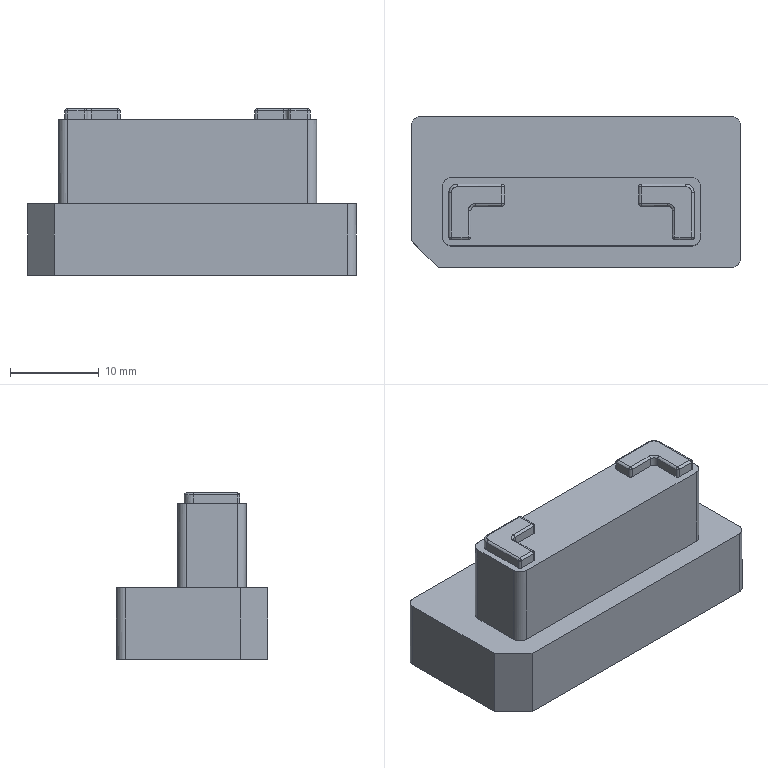NC program | PowerMill | posted with a generic post | part box 37 x 17 x 18.689 mm
Lines 3504 to 4371 of 30982:
N3601 M6
N3602 S18000 M03
N3603 G00 G90 X0.0 Y0.0
N3604 G43 Z9.7991 H2
N3605
N3606 G05 P10000 R4
N3607 X-17.264 Y-4.1178
N3608 Z0.7955
N3609 G01 Z-0.4045 F3600.0
N3610 X-17.2443 Y-4.1277 F6000.0
N3611 G03 X-16.9786 Y-4.0391 I0.0886 J0.1771
N3612 G01 X-16.3013 Y-2.6843
N3613 X-16.3014 Y-0.244
N3614 X-16.2791 Y0.244
N3615 X-16.1772 Y0.7321
N3616 X-15.9859 Y1.2201
N3617 X-15.6795 Y1.7082
N3618 X-15.2056 Y2.1962
N3619 X-14.6416 Y2.5601
N3620 X-14.1535 Y2.7484
N3621 X-13.6655 Y2.8465
N3622 X-13.1774 Y2.8715
N3623 X-8.2969 Y2.871
N3624 X-7.8088 Y2.8049
N3625 X-7.3208 Y2.6313
N3626 X-6.8327 Y2.3035
N3627 X-6.7176 Y2.1962
N3628 X-6.3488 Y1.7082
N3629 X-6.1463 Y1.2201
N3630 X-6.06 Y0.7321
N3631 X-6.0548 Y-1.2201
N3632 X-6.0876 Y-1.7082
N3633 X-6.2286 Y-2.1962
N3634 X-6.3447 Y-2.4359
N3635 X-6.5053 Y-2.6843
N3636 X-6.8327 Y-3.0394
N3637 X-7.0002 Y-3.1723
N3638 X-7.3208 Y-3.3669
N3639 X-7.8088 Y-3.5431
N3640 X-8.2969 Y-3.606
N3641 X-9.6235 Y-3.6064
N3642 G03 X-9.8185 Y-3.7754 I-0.0025 J-0.1942
N3643 G01 X-9.8234 Y-3.8064
N3644 X-9.8238 Y-5.1246
N3645 X-9.8882 Y-5.6126
N3646 X-10.0595 Y-6.1007
N3647 X-10.2491 Y-6.4163
N3648 X-10.3841 Y-6.5887
N3649 X-10.7372 Y-6.9154
N3650 X-10.9788 Y-7.0768
N3651 X-11.2252 Y-7.1978
N3652 X-11.7133 Y-7.3359
N3653 X-12.2013 Y-7.3752
N3654 X-14.1535 Y-7.3707
N3655 X-14.6416 Y-7.288
N3656 X-15.1461 Y-7.0768
N3657 X-15.6177 Y-6.7207
N3658 X-15.7419 Y-6.5887
N3659 X-16.0662 Y-6.1007
N3660 X-16.2402 Y-5.6126
N3661 X-16.3012 Y-5.1246
N3662 X-16.3013 Y-2.6843
N3663 X-17.264 Y-4.1178 Z-0.598
N3664 X-17.2443 Y-4.1277
N3665 G03 X-16.9787 Y-4.0391 I0.0885 J0.1771
N3666 G01 X-16.3013 Y-2.6843
N3667 X-16.3014 Y-0.244
N3668 X-16.2792 Y0.244
N3669 X-16.1773 Y0.7321
N3670 X-15.9859 Y1.2201
N3671 X-15.6795 Y1.7082
N3672 X-15.2056 Y2.1962
N3673 X-14.6416 Y2.5602
N3674 X-14.1535 Y2.7485
N3675 X-13.6655 Y2.8465
N3676 X-13.1774 Y2.8715
N3677 X-8.2969 Y2.871
N3678 X-7.8088 Y2.8049
N3679 X-7.3208 Y2.6314
N3680 X-6.8327 Y2.3035
N3681 X-6.7176 Y2.1962
N3682 X-6.3488 Y1.7082
N3683 X-6.1463 Y1.2201
N3684 X-6.06 Y0.7321
N3685 X-6.0548 Y-1.2201
N3686 X-6.0876 Y-1.7082
N3687 X-6.2286 Y-2.1962
N3688 X-6.3447 Y-2.436
N3689 X-6.5053 Y-2.6843
N3690 X-6.8327 Y-3.0394
N3691 X-7.0002 Y-3.1723
N3692 X-7.3208 Y-3.367
N3693 X-7.8088 Y-3.5432
N3694 X-8.2969 Y-3.6061
N3695 X-9.6235 Y-3.6064
N3696 G03 X-9.8185 Y-3.7754 I-0.0025 J-0.1942
N3697 G01 X-9.8234 Y-3.8064
N3698 X-9.8238 Y-5.1246
N3699 X-9.8882 Y-5.6126
N3700 X-10.0595 Y-6.1007
N3701 X-10.2491 Y-6.4163
N3702 X-10.3841 Y-6.5887
N3703 X-10.7372 Y-6.9154
N3704 X-10.9788 Y-7.0768
N3705 X-11.2252 Y-7.1978
N3706 X-11.7133 Y-7.3359
N3707 X-12.2013 Y-7.3752
N3708 X-14.1535 Y-7.3708
N3709 X-14.6416 Y-7.288
N3710 X-15.1461 Y-7.0768
N3711 X-15.6177 Y-6.7208
N3712 X-15.742 Y-6.5887
N3713 X-16.0662 Y-6.1007
N3714 X-16.2402 Y-5.6126
N3715 X-16.3012 Y-5.1246
N3716 X-16.3013 Y-2.6843
N3717 X-17.264 Y-4.1178 Z-0.7914
N3718 X-17.2443 Y-4.1277
N3719 G03 X-16.9787 Y-4.0391 I0.0885 J0.1771
N3720 G01 X-16.3014 Y-2.6843
N3721 X-16.3015 Y-0.244
N3722 X-16.2793 Y0.244
N3723 X-16.1773 Y0.7321
N3724 X-15.9859 Y1.2201
N3725 X-15.6795 Y1.7082
N3726 X-15.2056 Y2.1962
N3727 X-14.6416 Y2.5602
N3728 X-14.1535 Y2.7485
N3729 X-13.6655 Y2.8465
N3730 X-13.1774 Y2.8715
N3731 X-8.2969 Y2.8711
N3732 X-7.8088 Y2.8049
N3733 X-7.3208 Y2.6314
N3734 X-6.8327 Y2.3035
N3735 X-6.7176 Y2.1962
N3736 X-6.3487 Y1.7082
N3737 X-6.1463 Y1.2201
N3738 X-6.06 Y0.7321
N3739 X-6.0547 Y-1.2201
N3740 X-6.0875 Y-1.7082
N3741 X-6.2285 Y-2.1962
N3742 X-6.3447 Y-2.436
N3743 X-6.5053 Y-2.6843
N3744 X-6.8327 Y-3.0394
N3745 X-7.0002 Y-3.1723
N3746 X-7.3208 Y-3.367
N3747 X-7.8088 Y-3.5432
N3748 X-8.2969 Y-3.6061
N3749 X-9.6235 Y-3.6065
N3750 G03 X-9.8185 Y-3.7754 I-0.0025 J-0.1941
N3751 G01 X-9.8234 Y-3.8064
N3752 X-9.8237 Y-5.1246
N3753 X-9.8882 Y-5.6126
N3754 X-10.0594 Y-6.1007
N3755 X-10.2491 Y-6.4163
N3756 X-10.3841 Y-6.5887
N3757 X-10.7372 Y-6.9154
N3758 X-10.9788 Y-7.0768
N3759 X-11.2252 Y-7.1979
N3760 X-11.7133 Y-7.3359
N3761 X-12.2013 Y-7.3752
N3762 X-14.1535 Y-7.3708
N3763 X-14.6416 Y-7.288
N3764 X-15.1461 Y-7.0768
N3765 X-15.6177 Y-6.7208
N3766 X-15.742 Y-6.5887
N3767 X-16.0662 Y-6.1007
N3768 X-16.2402 Y-5.6126
N3769 X-16.3012 Y-5.1246
N3770 X-16.3014 Y-2.6843
N3771 X-17.264 Y-4.1178 Z-0.9849
N3772 X-17.2443 Y-4.1277
N3773 G03 X-16.9787 Y-4.0391 I0.0885 J0.1771
N3774 G01 X-16.3014 Y-2.6843
N3775 X-16.3015 Y-0.244
N3776 X-16.2795 Y0.244
N3777 X-16.1773 Y0.7321
N3778 X-15.986 Y1.2201
N3779 X-15.6795 Y1.7082
N3780 X-15.2056 Y2.1962
N3781 X-14.6416 Y2.5602
N3782 X-14.1535 Y2.7485
N3783 X-13.6655 Y2.8465
N3784 X-13.1774 Y2.8716
N3785 X-8.2969 Y2.8711
N3786 X-7.8088 Y2.8049
N3787 X-7.3208 Y2.6314
N3788 X-6.8327 Y2.3036
N3789 X-6.7176 Y2.1962
N3790 X-6.3487 Y1.7082
N3791 X-6.1462 Y1.2201
N3792 X-6.06 Y0.7321
N3793 X-6.0547 Y-1.2201
N3794 X-6.0875 Y-1.7082
N3795 X-6.2285 Y-2.1962
N3796 X-6.3447 Y-2.436
N3797 X-6.5053 Y-2.6843
N3798 X-6.8327 Y-3.0395
N3799 X-7.0001 Y-3.1723
N3800 X-7.3208 Y-3.367
N3801 X-7.8088 Y-3.5432
N3802 X-8.2969 Y-3.6061
N3803 X-9.6235 Y-3.6065
N3804 G03 X-9.8185 Y-3.7754 I-0.0025 J-0.1941
N3805 G01 X-9.8234 Y-3.8064
N3806 X-9.8237 Y-5.1246
N3807 X-9.8882 Y-5.6126
N3808 X-10.0594 Y-6.1007
N3809 X-10.2491 Y-6.4163
N3810 X-10.384 Y-6.5887
N3811 X-10.7372 Y-6.9154
N3812 X-10.9788 Y-7.0768
N3813 X-11.2252 Y-7.1979
N3814 X-11.7133 Y-7.336
N3815 X-12.2013 Y-7.3752
N3816 X-14.1535 Y-7.3708
N3817 X-14.6416 Y-7.2881
N3818 X-15.1461 Y-7.0768
N3819 X-15.6177 Y-6.7208
N3820 X-15.742 Y-6.5887
N3821 X-16.0663 Y-6.1007
N3822 X-16.2403 Y-5.6126
N3823 X-16.3013 Y-5.1246
N3824 X-16.3014 Y-2.6843
N3825 X-17.264 Y-4.1178 Z-1.1784
N3826 X-17.2444 Y-4.1276
N3827 G03 X-16.9787 Y-4.0391 I0.0886 J0.1771
N3828 G01 X-16.3014 Y-2.6843
N3829 X-16.3015 Y-0.244
N3830 X-16.2796 Y0.244
N3831 X-16.1773 Y0.7321
N3832 X-15.986 Y1.2201
N3833 X-15.6796 Y1.7082
N3834 X-15.2056 Y2.1962
N3835 X-14.6416 Y2.5602
N3836 X-14.1535 Y2.7485
N3837 X-13.6655 Y2.8466
N3838 X-13.1774 Y2.8716
N3839 X-8.2969 Y2.8711
N3840 X-7.8088 Y2.805
N3841 X-7.3208 Y2.6314
N3842 X-6.8327 Y2.3036
N3843 X-6.7175 Y2.1962
N3844 X-6.3487 Y1.7082
N3845 X-6.1462 Y1.2201
N3846 X-6.06 Y0.7321
N3847 X-6.0547 Y-1.2201
N3848 X-6.0875 Y-1.7082
N3849 X-6.2285 Y-2.1962
N3850 X-6.3447 Y-2.436
N3851 X-6.5052 Y-2.6843
N3852 X-6.8327 Y-3.0395
N3853 X-7.0001 Y-3.1723
N3854 X-7.3208 Y-3.367
N3855 X-7.8088 Y-3.5432
N3856 X-8.2969 Y-3.6061
N3857 X-9.6235 Y-3.6065
N3858 G03 X-9.8185 Y-3.7754 I-0.0025 J-0.1941
N3859 G01 X-9.8234 Y-3.8064
N3860 X-9.8237 Y-5.1246
N3861 X-9.8882 Y-5.6126
N3862 X-10.0594 Y-6.1007
N3863 X-10.2491 Y-6.4163
N3864 X-10.384 Y-6.5887
N3865 X-10.7372 Y-6.9155
N3866 X-10.9788 Y-7.0768
N3867 X-11.2252 Y-7.1979
N3868 X-11.7133 Y-7.336
N3869 X-12.2013 Y-7.3753
N3870 X-14.1535 Y-7.3708
N3871 X-14.6416 Y-7.2881
N3872 X-15.1462 Y-7.0768
N3873 X-15.6177 Y-6.7208
N3874 X-15.742 Y-6.5887
N3875 X-16.0663 Y-6.1007
N3876 X-16.2403 Y-5.6126
N3877 X-16.3013 Y-5.1246
N3878 X-16.3014 Y-2.6843
N3879 X-17.3042 Y-4.1981 Z-1.3719
N3880 X-17.2845 Y-4.208
N3881 G03 X-17.0189 Y-4.1194 I0.0885 J0.1771
N3882 G01 X-16.3014 Y-2.6843
N3883 X-16.3015 Y-0.244
N3884 X-16.2796 Y0.244
N3885 X-16.1774 Y0.7321
N3886 X-15.986 Y1.2201
N3887 X-15.6796 Y1.7082
N3888 X-15.2057 Y2.1962
N3889 X-14.6416 Y2.5602
N3890 X-14.1535 Y2.7485
N3891 X-13.6655 Y2.8466
N3892 X-13.1774 Y2.8716
N3893 X-8.2969 Y2.8711
N3894 X-7.8088 Y2.805
N3895 X-7.3208 Y2.6314
N3896 X-6.8327 Y2.3036
N3897 X-6.7175 Y2.1962
N3898 X-6.3487 Y1.7082
N3899 X-6.1462 Y1.2201
N3900 X-6.0599 Y0.7321
N3901 X-6.0547 Y-1.2201
N3902 X-6.0875 Y-1.7082
N3903 X-6.2285 Y-2.1962
N3904 X-6.3447 Y-2.4361
N3905 X-6.5052 Y-2.6843
N3906 X-6.8327 Y-3.0395
N3907 X-7.0001 Y-3.1723
N3908 X-7.3208 Y-3.3671
N3909 X-7.8088 Y-3.5433
N3910 X-8.2969 Y-3.6061
N3911 X-9.6235 Y-3.6065
N3912 G03 X-9.8234 Y-3.8064 I0.0001 J-0.2
N3913 G01 X-9.8237 Y-5.1246
N3914 X-9.8881 Y-5.6126
N3915 X-10.0594 Y-6.1007
N3916 X-10.2491 Y-6.4164
N3917 X-10.384 Y-6.5887
N3918 X-10.7372 Y-6.9155
N3919 X-10.9787 Y-7.0768
N3920 X-11.2252 Y-7.1979
N3921 X-11.7133 Y-7.336
N3922 X-12.2013 Y-7.3753
N3923 X-14.1535 Y-7.3709
N3924 X-14.6416 Y-7.2881
N3925 X-15.1296 Y-7.0861
N3926 X-15.1378 Y-7.0812
N3927 X-15.1461 Y-7.0767
N3928 X-15.6045 Y-6.7307
N3929 X-15.6177 Y-6.7208
N3930 X-15.742 Y-6.5887
N3931 X-16.0663 Y-6.1007
N3932 X-16.2403 Y-5.6126
N3933 X-16.3013 Y-5.1246
N3934 X-16.3014 Y-2.6843
N3935 G00 Z3.7955
N3936 G01 X4.2528 Y-2.3244 F10000.0
N3937 G00 Z0.7955
N3938 G01 Z-0.4045 F3600.0
N3939 X4.2725 Y-2.3343 F6000.0
N3940 G03 X4.5384 Y-2.2464 I0.089 J0.1769
N3941 G01 X5.0547 Y-1.2201
N3942 X5.0597 Y0.7321
N3943 X5.1446 Y1.2201
N3944 X5.3488 Y1.7082
N3945 X5.7177 Y2.1962
N3946 X5.8566 Y2.3251
N3947 X6.3447 Y2.6436
N3948 X6.8327 Y2.814
N3949 X7.3208 Y2.8713
N3950 X12.2013 Y2.8715
N3951 X12.6894 Y2.8441
N3952 X13.1774 Y2.7408
N3953 X13.6655 Y2.548
N3954 X14.1535 Y2.2375
N3955 X14.6416 Y1.7566
N3956 X14.9859 Y1.2201
N3957 X15.1296 Y0.882
N3958 X15.2796 Y0.244
N3959 X15.3014 Y-0.244
N3960 X15.3012 Y-5.1246
N3961 X15.2367 Y-5.6126
N3962 X15.0656 Y-6.1007
N3963 X14.7409 Y-6.5887
N3964 X14.6416 Y-6.6969
N3965 X14.1462 Y-7.0768
N3966 X13.6655 Y-7.2794
N3967 X13.1774 Y-7.3688
N3968 X11.2252 Y-7.3752
N3969 X10.7372 Y-7.3449
N3970 X10.2491 Y-7.2077
N3971 X9.9789 Y-7.0768
N3972 X9.7611 Y-6.936
N3973 X9.3832 Y-6.5887
N3974 X9.273 Y-6.4511
N3975 X9.0588 Y-6.1007
N3976 X8.8848 Y-5.6126
N3977 X8.8238 Y-5.1246
N3978 X8.8235 Y-3.8065
N3979 G03 X8.6081 Y-3.6065 I-0.201 J-0.0005
N3980 G01 X7.3208 Y-3.6064
N3981 X6.8327 Y-3.5449
N3982 X6.3447 Y-3.3781
N3983 X6.0022 Y-3.1723
N3984 X5.8566 Y-3.0588
N3985 X5.5081 Y-2.6843
N3986 X5.3686 Y-2.4777
N3987 X5.2286 Y-2.1962
N3988 X5.0923 Y-1.7082
N3989 X5.0547 Y-1.2201
N3990 X2.7752 Y1.805 Z-0.298
N3991 X2.6121 Y1.6908 Z-0.3014 F3600.0
N3992 X2.1438 Y1.2225 Z-0.313
N3993 X1.7638 Y0.6799 Z-0.3246
N3994 X1.4839 Y0.0795 Z-0.3361
N3995 X1.3125 Y-0.5603 Z-0.3477
N3996 X1.2547 Y-1.2201 Z-0.3592
N3997 X1.3125 Y-1.88 Z-0.3708
N3998 X1.4839 Y-2.5198 Z-0.3824
N3999 X1.7638 Y-3.1201 Z-0.3939
N4000 X2.1438 Y-3.6627 Z-0.4055
N4001 X2.6121 Y-4.1311 Z-0.417
N4002 X3.1547 Y-4.511 Z-0.4286
N4003 X3.7551 Y-4.791 Z-0.4402
N4004 X4.3949 Y-4.9624 Z-0.4517
N4005 X5.0547 Y-5.0201 Z-0.4633
N4006 X5.7146 Y-4.9624 Z-0.4748
N4007 X6.3544 Y-4.791 Z-0.4864
N4008 X6.9547 Y-4.511 Z-0.498
N4009 X7.4973 Y-4.1311 Z-0.5095
N4010 X7.9657 Y-3.6627 Z-0.5211
N4011 X7.9841 Y-3.6365 Z-0.5216
N4012 X7.3208 Y-3.6364 Z-0.5332
N4013 X7.317 Y-3.6362 Z-0.5333
N4014 X6.829 Y-3.5747 Z-0.5419
N4015 X6.823 Y-3.5733 Z-0.542
N4016 X6.335 Y-3.4065 Z-0.551
N4017 X6.3292 Y-3.4039 Z-0.5511
N4018 X5.9867 Y-3.1981 Z-0.558
N4019 X5.9837 Y-3.196 Z-0.5581
N4020 X5.8382 Y-3.0825 Z-0.5613
N4021 X5.8347 Y-3.0792 Z-0.5614
N4022 X5.4861 Y-2.7047 Z-0.5703
N4023 X5.4832 Y-2.7011 Z-0.5704
N4024 X5.3437 Y-2.4945 Z-0.5748
N4025 X5.3417 Y-2.4911
N4026 X5.2017 Y-2.2096 Z-0.5803
N4027 X5.1997 Y-2.2043 Z-0.5804
N4028 X5.0634 Y-1.7163 Z-0.5893
N4029 X5.0624 Y-1.7105 Z-0.5894
N4030 X5.0248 Y-1.2224 Z-0.5979
N4031 X5.0247 Y-1.2201 Z-0.598
N4032 X5.0547
N4033 X5.0597 Y0.7321 F6000.0
N4034 X5.1445 Y1.2201
N4035 X5.3488 Y1.7082
N4036 X5.7176 Y2.1962
N4037 X5.8566 Y2.3251
N4038 X6.3447 Y2.6437
N4039 X6.8327 Y2.814
N4040 X7.3208 Y2.8714
N4041 X12.2013 Y2.8715
N4042 X12.6894 Y2.8441
N4043 X13.1774 Y2.7408
N4044 X13.6655 Y2.548
N4045 X14.1535 Y2.2375
N4046 X14.6416 Y1.7566
N4047 X14.986 Y1.2201
N4048 X15.1296 Y0.882
N4049 X15.2796 Y0.244
N4050 X15.3015 Y-0.244
N4051 X15.3012 Y-5.1246
N4052 X15.2367 Y-5.6126
N4053 X15.0656 Y-6.1007
N4054 X14.7409 Y-6.5887
N4055 X14.6416 Y-6.697
N4056 X14.1462 Y-7.0768
N4057 X13.6655 Y-7.2794
N4058 X13.1774 Y-7.3688
N4059 X11.2252 Y-7.3752
N4060 X10.7372 Y-7.3449
N4061 X10.2491 Y-7.2077
N4062 X9.9789 Y-7.0768
N4063 X9.7611 Y-6.936
N4064 X9.3831 Y-6.5887
N4065 X9.273 Y-6.4512
N4066 X9.0588 Y-6.1007
N4067 X8.8847 Y-5.6126
N4068 X8.8238 Y-5.1246
N4069 X8.8235 Y-3.8065
N4070 G03 X8.6081 Y-3.6065 I-0.201 J-0.0005
N4071 G01 X7.3208 Y-3.6064
N4072 X6.8327 Y-3.545
N4073 X6.3447 Y-3.3782
N4074 X6.0022 Y-3.1723
N4075 X5.8566 Y-3.0588
N4076 X5.508 Y-2.6843
N4077 X5.3686 Y-2.4777
N4078 X5.2286 Y-2.1962
N4079 X5.0923 Y-1.7082
N4080 X5.0547 Y-1.2201
N4081 X2.7752 Y1.805 Z-0.4914
N4082 X2.6121 Y1.6908 Z-0.4949 F3600.0
N4083 X2.1437 Y1.2225 Z-0.5065
N4084 X1.7638 Y0.6799 Z-0.518
N4085 X1.4839 Y0.0795 Z-0.5296
N4086 X1.3124 Y-0.5603 Z-0.5412
N4087 X1.2547 Y-1.2201 Z-0.5527
N4088 X1.3124 Y-1.88 Z-0.5643
N4089 X1.4839 Y-2.5198 Z-0.5758
N4090 X1.7638 Y-3.1201 Z-0.5874
N4091 X2.1437 Y-3.6627 Z-0.599
N4092 X2.6121 Y-4.1311 Z-0.6105
N4093 X3.1547 Y-4.511 Z-0.6221
N4094 X3.755 Y-4.791 Z-0.6336
N4095 X4.3948 Y-4.9624 Z-0.6452
N4096 X5.0547 Y-5.0201 Z-0.6568
N4097 X5.7146 Y-4.9624 Z-0.6683
N4098 X6.3544 Y-4.791 Z-0.6799
N4099 X6.9547 Y-4.511 Z-0.6914
N4100 X7.4973 Y-4.1311 Z-0.703
N4101 X7.9657 Y-3.6627 Z-0.7146
N4102 X7.9841 Y-3.6365 Z-0.7151
N4103 X7.3208 Y-3.6364 Z-0.7267
N4104 X7.317 Y-3.6362 Z-0.7268
N4105 X6.829 Y-3.5747 Z-0.7353
N4106 X6.823 Y-3.5734 Z-0.7354
N4107 X6.335 Y-3.4066 Z-0.7444
N4108 X6.3292 Y-3.4039 Z-0.7446
N4109 X5.9867 Y-3.1981 Z-0.7515
N4110 X5.9837 Y-3.196 Z-0.7516
N4111 X5.8382 Y-3.0825 Z-0.7548
N4112 X5.8347 Y-3.0793 Z-0.7549
N4113 X5.4861 Y-2.7047 Z-0.7638
N4114 X5.4832 Y-2.7011 Z-0.7639
N4115 X5.3437 Y-2.4945 Z-0.7683
N4116 X5.3417 Y-2.4911
N4117 X5.2017 Y-2.2096 Z-0.7738
N4118 X5.1996 Y-2.2043 Z-0.7739
N4119 X5.0634 Y-1.7163 Z-0.7828
N4120 X5.0624 Y-1.7105 Z-0.7829
N4121 X5.0248 Y-1.2224 Z-0.7914
N4122 X5.0247 Y-1.2201
N4123 X5.0324 Y-1.2126
N4124 X5.0397 Y-1.2204
N4125 X5.0473 Y-1.2282
N4126 X5.0547 Y-1.2201
N4127 X5.0596 Y0.7321 F6000.0
N4128 X5.1445 Y1.2201
N4129 X5.3487 Y1.7082
N4130 X5.7176 Y2.1962
N4131 X5.8566 Y2.3251
N4132 X6.3447 Y2.6437
N4133 X6.8327 Y2.814
N4134 X7.3208 Y2.8714
N4135 X12.2013 Y2.8715
N4136 X12.6894 Y2.8441
N4137 X13.1774 Y2.7408
N4138 X13.6655 Y2.5481
N4139 X14.1535 Y2.2375
N4140 X14.6416 Y1.7567
N4141 X14.986 Y1.2201
N4142 X15.1296 Y0.8821
N4143 X15.2796 Y0.244
N4144 X15.3015 Y-0.244
N4145 X15.3012 Y-5.1246
N4146 X15.2367 Y-5.6126
N4147 X15.0656 Y-6.1007
N4148 X14.7409 Y-6.5887
N4149 X14.6416 Y-6.697
N4150 X14.1462 Y-7.0768
N4151 X13.6655 Y-7.2794
N4152 X13.1774 Y-7.3688
N4153 X11.2252 Y-7.3752
N4154 X10.7372 Y-7.345
N4155 X10.2491 Y-7.2077
N4156 X9.9789 Y-7.0768
N4157 X9.7611 Y-6.936
N4158 X9.3831 Y-6.5887
N4159 X9.273 Y-6.4512
N4160 X9.0588 Y-6.1007
N4161 X8.8847 Y-5.6126
N4162 X8.8238 Y-5.1246
N4163 X8.8235 Y-3.8065
N4164 G03 X8.608 Y-3.6065 I-0.201 J-0.0005
N4165 G01 X7.3208 Y-3.6064
N4166 X6.8327 Y-3.545
N4167 X6.3447 Y-3.3782
N4168 X6.0021 Y-3.1723
N4169 X5.8566 Y-3.0588
N4170 X5.508 Y-2.6843
N4171 X5.3686 Y-2.4777
N4172 X5.2285 Y-2.1962
N4173 X5.0923 Y-1.7082
N4174 X5.0547 Y-1.2201
N4175 X2.7752 Y1.805 Z-0.6849
N4176 X2.6121 Y1.6908 Z-0.6884 F3600.0
N4177 X2.1437 Y1.2225 Z-0.7
N4178 X1.7638 Y0.6799 Z-0.7115
N4179 X1.4839 Y0.0795 Z-0.7231
N4180 X1.3124 Y-0.5603 Z-0.7346
N4181 X1.2547 Y-1.2201 Z-0.7462
N4182 X1.3124 Y-1.88 Z-0.7578
N4183 X1.4839 Y-2.5198 Z-0.7693
N4184 X1.7638 Y-3.1201 Z-0.7809
N4185 X2.1437 Y-3.6627 Z-0.7924
N4186 X2.6121 Y-4.1311 Z-0.804
N4187 X3.1547 Y-4.511 Z-0.8156
N4188 X3.755 Y-4.791 Z-0.8271
N4189 X4.3948 Y-4.9624 Z-0.8387
N4190 X5.0547 Y-5.0201 Z-0.8502
N4191 X5.7146 Y-4.9624 Z-0.8618
N4192 X6.3544 Y-4.791 Z-0.8734
N4193 X6.9547 Y-4.511 Z-0.8849
N4194 X7.4973 Y-4.1311 Z-0.8965
N4195 X7.9657 Y-3.6627 Z-0.908
N4196 X7.984 Y-3.6365 Z-0.9086
N4197 X7.3208 Y-3.6364 Z-0.9202
N4198 X7.317 Y-3.6362
N4199 X6.829 Y-3.5748 Z-0.9288
N4200 X6.823 Y-3.5734 Z-0.9289
N4201 X6.335 Y-3.4066 Z-0.9379
N4202 X6.3292 Y-3.4039 Z-0.938
N4203 X5.9867 Y-3.1981 Z-0.945
N4204 X5.9837 Y-3.196 Z-0.9451
N4205 X5.8382 Y-3.0825 Z-0.9483
N4206 X5.8347 Y-3.0793 Z-0.9484
N4207 X5.486 Y-2.7047 Z-0.9573
N4208 X5.4831 Y-2.7011 Z-0.9574
N4209 X5.3437 Y-2.4945 Z-0.9617
N4210 X5.3417 Y-2.4911 Z-0.9618
N4211 X5.2017 Y-2.2096 Z-0.9673
N4212 X5.1996 Y-2.2043 Z-0.9674
N4213 X5.0634 Y-1.7163 Z-0.9762
N4214 X5.0624 Y-1.7105 Z-0.9763
N4215 X5.0248 Y-1.2224 Z-0.9849
N4216 X5.0247 Y-1.2201
N4217 X5.0324 Y-1.2126
N4218 X5.0397 Y-1.2204
N4219 X5.0473 Y-1.2282
N4220 X5.0547 Y-1.2201
N4221 X5.0596 Y0.7321 F6000.0
N4222 X5.1445 Y1.2201
N4223 X5.3487 Y1.7082
N4224 X5.7176 Y2.1962
N4225 X5.8566 Y2.3251
N4226 X6.3447 Y2.6437
N4227 X6.8327 Y2.814
N4228 X7.3208 Y2.8714
N4229 X12.2013 Y2.8716
N4230 X12.6894 Y2.8442
N4231 X13.1774 Y2.7409
N4232 X13.6655 Y2.5481
N4233 X14.1535 Y2.2375
N4234 X14.6416 Y1.7567
N4235 X14.986 Y1.2201
N4236 X15.1296 Y0.8821
N4237 X15.2796 Y0.244
N4238 X15.3015 Y-0.244
N4239 X15.3012 Y-5.1246
N4240 X15.2368 Y-5.6126
N4241 X15.0656 Y-6.1007
N4242 X14.7409 Y-6.5887
N4243 X14.6416 Y-6.697
N4244 X14.1462 Y-7.0768
N4245 X13.6655 Y-7.2795
N4246 X13.1774 Y-7.3688
N4247 X11.2252 Y-7.3752
N4248 X10.7372 Y-7.345
N4249 X10.2491 Y-7.2078
N4250 X9.9789 Y-7.0768
N4251 X9.7611 Y-6.9361
N4252 X9.3831 Y-6.5887
N4253 X9.273 Y-6.4512
N4254 X9.0588 Y-6.1007
N4255 X8.8847 Y-5.6126
N4256 X8.8238 Y-5.1246
N4257 X8.8235 Y-3.8065
N4258 G03 X8.608 Y-3.6065 I-0.201 J-0.0005
N4259 G01 X7.3208 Y-3.6064
N4260 X6.8327 Y-3.545
N4261 X6.3447 Y-3.3782
N4262 X6.0021 Y-3.1723
N4263 X5.8566 Y-3.0588
N4264 X5.508 Y-2.6843
N4265 X5.3686 Y-2.4778
N4266 X5.2285 Y-2.1962
N4267 X5.0923 Y-1.7082
N4268 X5.0547 Y-1.2201
N4269 X2.7771 Y1.8064 Z-0.8784
N4270 X2.6121 Y1.6908 Z-0.8819 F3600.0
N4271 X2.1437 Y1.2225 Z-0.8935
N4272 X1.7638 Y0.6799 Z-0.905
N4273 X1.4838 Y0.0795 Z-0.9166
N4274 X1.3124 Y-0.5603 Z-0.9282
N4275 X1.2547 Y-1.2201 Z-0.9397
N4276 X1.3124 Y-1.88 Z-0.9513
N4277 X1.4838 Y-2.5198 Z-0.9628
N4278 X1.7638 Y-3.1201 Z-0.9744
N4279 X2.1437 Y-3.6627 Z-0.986
N4280 X2.6121 Y-4.1311 Z-0.9975
N4281 X3.1547 Y-4.511 Z-1.0091
N4282 X3.755 Y-4.791 Z-1.0206
N4283 X4.3948 Y-4.9624 Z-1.0322
N4284 X5.0547 Y-5.0201 Z-1.0438
N4285 X5.7145 Y-4.9624 Z-1.0553
N4286 X6.3543 Y-4.791 Z-1.0669
N4287 X6.9547 Y-4.511 Z-1.0784
N4288 X7.4973 Y-4.1311 Z-1.09
N4289 X7.9656 Y-3.6627 Z-1.1016
N4290 X7.984 Y-3.6365 Z-1.1021
N4291 X7.3208 Z-1.1137
N4292 X7.317 Y-3.6362 Z-1.1138
N4293 X6.829 Y-3.5748 Z-1.1223
N4294 X6.823 Y-3.5734 Z-1.1224
N4295 X6.335 Y-3.4066 Z-1.1314
N4296 X6.3292 Y-3.4039 Z-1.1316
N4297 X5.9867 Y-3.1981 Z-1.1385
N4298 X5.9837 Y-3.196 Z-1.1386
N4299 X5.8382 Y-3.0825 Z-1.1418
N4300 X5.8347 Y-3.0793 Z-1.1419
N4301 X5.486 Y-2.7047 Z-1.1508
N4302 X5.4831 Y-2.7011 Z-1.1509
N4303 X5.3437 Y-2.4946 Z-1.1553
N4304 X5.3417 Y-2.4911
N4305 X5.2016 Y-2.2096 Z-1.1608
N4306 X5.1996 Y-2.2043 Z-1.1609
N4307 X5.0634 Y-1.7163 Z-1.1698
N4308 X5.0623 Y-1.7105 Z-1.1699
N4309 X5.0248 Y-1.2224 Z-1.1784
N4310 X5.0317 Y-1.2144
N4311 X5.0397 Y-1.2213
N4312 X5.0478 Y-1.2282
N4313 X5.0547 Y-1.2201
N4314 X5.0596 Y0.7321 F6000.0
N4315 X5.1445 Y1.2201
N4316 X5.3487 Y1.7082
N4317 X5.7176 Y2.1962
N4318 X5.8566 Y2.3251
N4319 X6.3447 Y2.6437
N4320 X6.8327 Y2.8141
N4321 X7.3208 Y2.8714
N4322 X12.2013 Y2.8716
N4323 X12.6894 Y2.8442
N4324 X13.1774 Y2.7409
N4325 X13.6655 Y2.5481
N4326 X14.1535 Y2.2376
N4327 X14.6416 Y1.7567
N4328 X14.986 Y1.2201
N4329 X15.1296 Y0.8821
N4330 X15.2797 Y0.244
N4331 X15.3015 Y-0.244
N4332 X15.3012 Y-5.1246
N4333 X15.2368 Y-5.6126
N4334 X15.0656 Y-6.1007
N4335 X14.741 Y-6.5887
N4336 X14.6416 Y-6.697
N4337 X14.1462 Y-7.0768
N4338 X13.6655 Y-7.2795
N4339 X13.1774 Y-7.3688
N4340 X11.2252 Y-7.3753
N4341 X10.7372 Y-7.345
N4342 X10.2491 Y-7.2078
N4343 X9.9788 Y-7.0768
N4344 X9.7611 Y-6.9361
N4345 X9.3831 Y-6.5887
N4346 X9.273 Y-6.4512
N4347 X9.0587 Y-6.1007
N4348 X8.8847 Y-5.6126
N4349 X8.8237 Y-5.1246
N4350 X8.8235 Y-3.8065
N4351 G03 X8.608 Y-3.6065 I-0.201 J-0.0005
N4352 G01 X7.3208
N4353 X6.8327 Y-3.545
N4354 X6.3447 Y-3.3782
N4355 X6.0021 Y-3.1723
N4356 X5.8566 Y-3.0589
N4357 X5.508 Y-2.6843
N4358 X5.3686 Y-2.4778
N4359 X5.2285 Y-2.1962
N4360 X5.0922 Y-1.7082
N4361 X5.0547 Y-1.2201
N4362 X2.7752 Y1.8051 Z-1.0719
N4363 X2.6121 Y1.6908 Z-1.0754 F3600.0
N4364 X2.1437 Y1.2225 Z-1.0869
N4365 X1.7638 Y0.6799 Z-1.0985
N4366 X1.4838 Y0.0795 Z-1.11
N4367 X1.3124 Y-0.5603 Z-1.1216
N4368 X1.2546 Y-1.2201 Z-1.1332
N4369 X1.3124 Y-1.88 Z-1.1447
N4370 X1.4838 Y-2.5198 Z-1.1563
N4371 X1.7638 Y-3.1201 Z-1.1678
N4372 X2.1437 Y-3.6627 Z-1.1794
N4373 X2.6121 Y-4.1311 Z-1.191
N4374 X3.1546 Y-4.511 Z-1.2025
N4375 X3.755 Y-4.791 Z-1.2141
N4376 X4.3948 Y-4.9624 Z-1.2256
N4377 X5.0546 Y-5.0201 Z-1.2372
N4378 X5.7145 Y-4.9624 Z-1.2488
N4379 X6.3543 Y-4.791 Z-1.2603
N4380 X6.9546 Y-4.511 Z-1.2719
N4381 X7.4972 Y-4.1311 Z-1.2834
N4382 X7.9656 Y-3.6627 Z-1.295
N4383 X7.984 Y-3.6365 Z-1.2955
N4384 X7.3208 Z-1.3071
N4385 X7.317 Y-3.6362 Z-1.3072
N4386 X6.829 Y-3.5748 Z-1.3158
N4387 X6.823 Y-3.5734 Z-1.3159
N4388 X6.335 Y-3.4066 Z-1.3249
N4389 X6.3292 Y-3.404 Z-1.325
N4390 X5.9866 Y-3.1981 Z-1.332
N4391 X5.9836 Y-3.196
N4392 X5.8382 Y-3.0826 Z-1.3353
N4393 X5.8347 Y-3.0793
N4394 X5.486 Y-2.7047 Z-1.3443
N4395 X5.4831 Y-2.7011
N4396 X5.3437 Y-2.4946 Z-1.3487
N4397 X5.3417 Y-2.4912 Z-1.3488
N4398 X5.2016 Y-2.2096 Z-1.3543
N4399 X5.1996 Y-2.2043 Z-1.3544
N4400 X5.0633 Y-1.7163 Z-1.3632
N4401 X5.0623 Y-1.7105 Z-1.3633
N4402 X5.0247 Y-1.2224 Z-1.3718
N4403 X5.0246 Y-1.2201 Z-1.3719
N4404 X5.0546
N4405 X5.0596 Y0.7321 F6000.0
N4406 X5.1445 Y1.2201
N4407 X5.3487 Y1.7082
N4408 X5.7175 Y2.1962
N4409 X5.8566 Y2.3252
N4410 X6.3447 Y2.6438
N4411 X6.8327 Y2.8141
N4412 X7.3208 Y2.8715
N4413 X12.2013 Y2.8716
N4414 X12.6894 Y2.8442
N4415 X13.1774 Y2.7409
N4416 X13.6655 Y2.5481
N4417 X14.1535 Y2.2376
N4418 X14.6416 Y1.7567
N4419 X14.9861 Y1.2201
N4420 X15.1296 Y0.8821
N4421 X15.2797 Y0.244
N4422 X15.3016 Y-0.244
N4423 X15.3013 Y-5.1246
N4424 X15.2368 Y-5.6126
N4425 X15.0657 Y-6.1007
N4426 X14.741 Y-6.5887
N4427 X14.6416 Y-6.697
N4428 X14.1463 Y-7.0768
N4429 X13.6655 Y-7.2795
N4430 X13.1774 Y-7.3689
N4431 X11.2252 Y-7.3753
N4432 X10.7372 Y-7.345
N4433 X10.2491 Y-7.2078
N4434 X9.9788 Y-7.0768
N4435 X9.7611 Y-6.9361
N4436 X9.3831 Y-6.5887
N4437 X9.273 Y-6.4512
N4438 X9.0587 Y-6.1007
N4439 X8.8846 Y-5.6126
N4440 X8.8237 Y-5.1246
N4441 X8.8235 Y-3.8065
N4442 G03 X8.608 Y-3.6065 I-0.201 J-0.0006
N4443 G01 X7.3208
N4444 X6.8327 Y-3.545
N4445 X6.3447 Y-3.3782
N4446 X6.0021 Y-3.1723
N4447 X5.8566 Y-3.0589
N4448 X5.5079 Y-2.6843
N4449 X5.3686 Y-2.4778
N4450 X5.2285 Y-2.1962
N4451 X5.0922 Y-1.7082
N4452 X5.0546 Y-1.2201
N4453 G00 Z9.7991
N4454 G05 P0
N4455 (---------------)
N4456 ( END TOOLPATH : 精公再粗02-外形偏置-D4C )
N4457 (---------------)
N4458
N4459 M05
N4460 G53 Z0.0
N4461 (---------------)
N4462 ( START TOOLPATH : 精公基准台01-平坦面平行-D10 )
N4463 (---------------)
N4464 ( TOOL NO.    :3 )
N4465 ( TOOL TYPE   : ENDMILL)
N4466 ( TOOL ID     : D10_1_1_1)
N4467 ( TOOL DIA    : 10.0 LENGTH 73.84)
N4468 T3